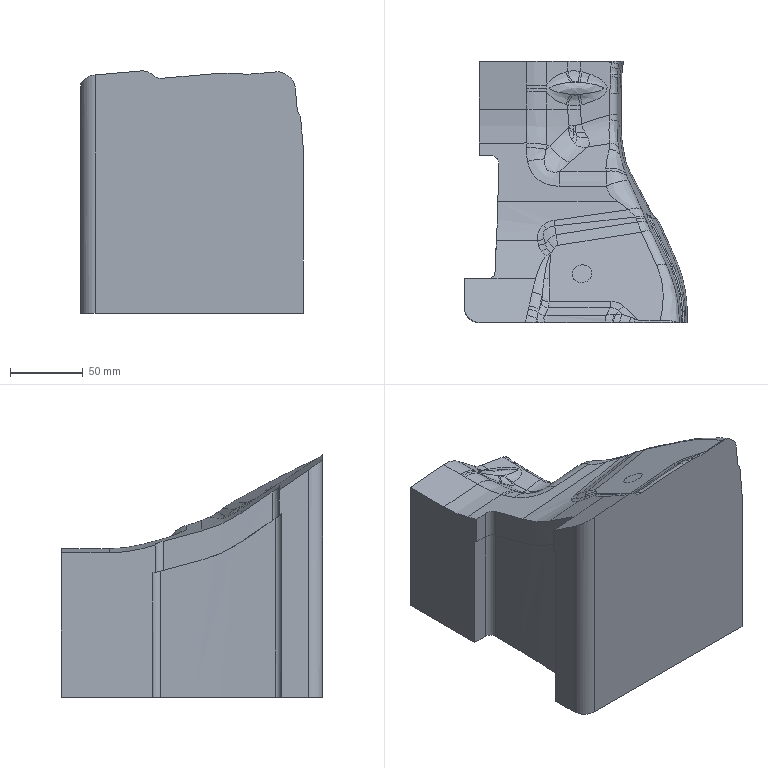Part | NX | features solid 2 | 1 solid | 169 faces | box 153.73 x 180.001 x 167.039 mm | volume 2430238 mm3 | spline 154 | plane 9 | cylinder 6 | commonest cylinder face diameters 10 x4 20 x2